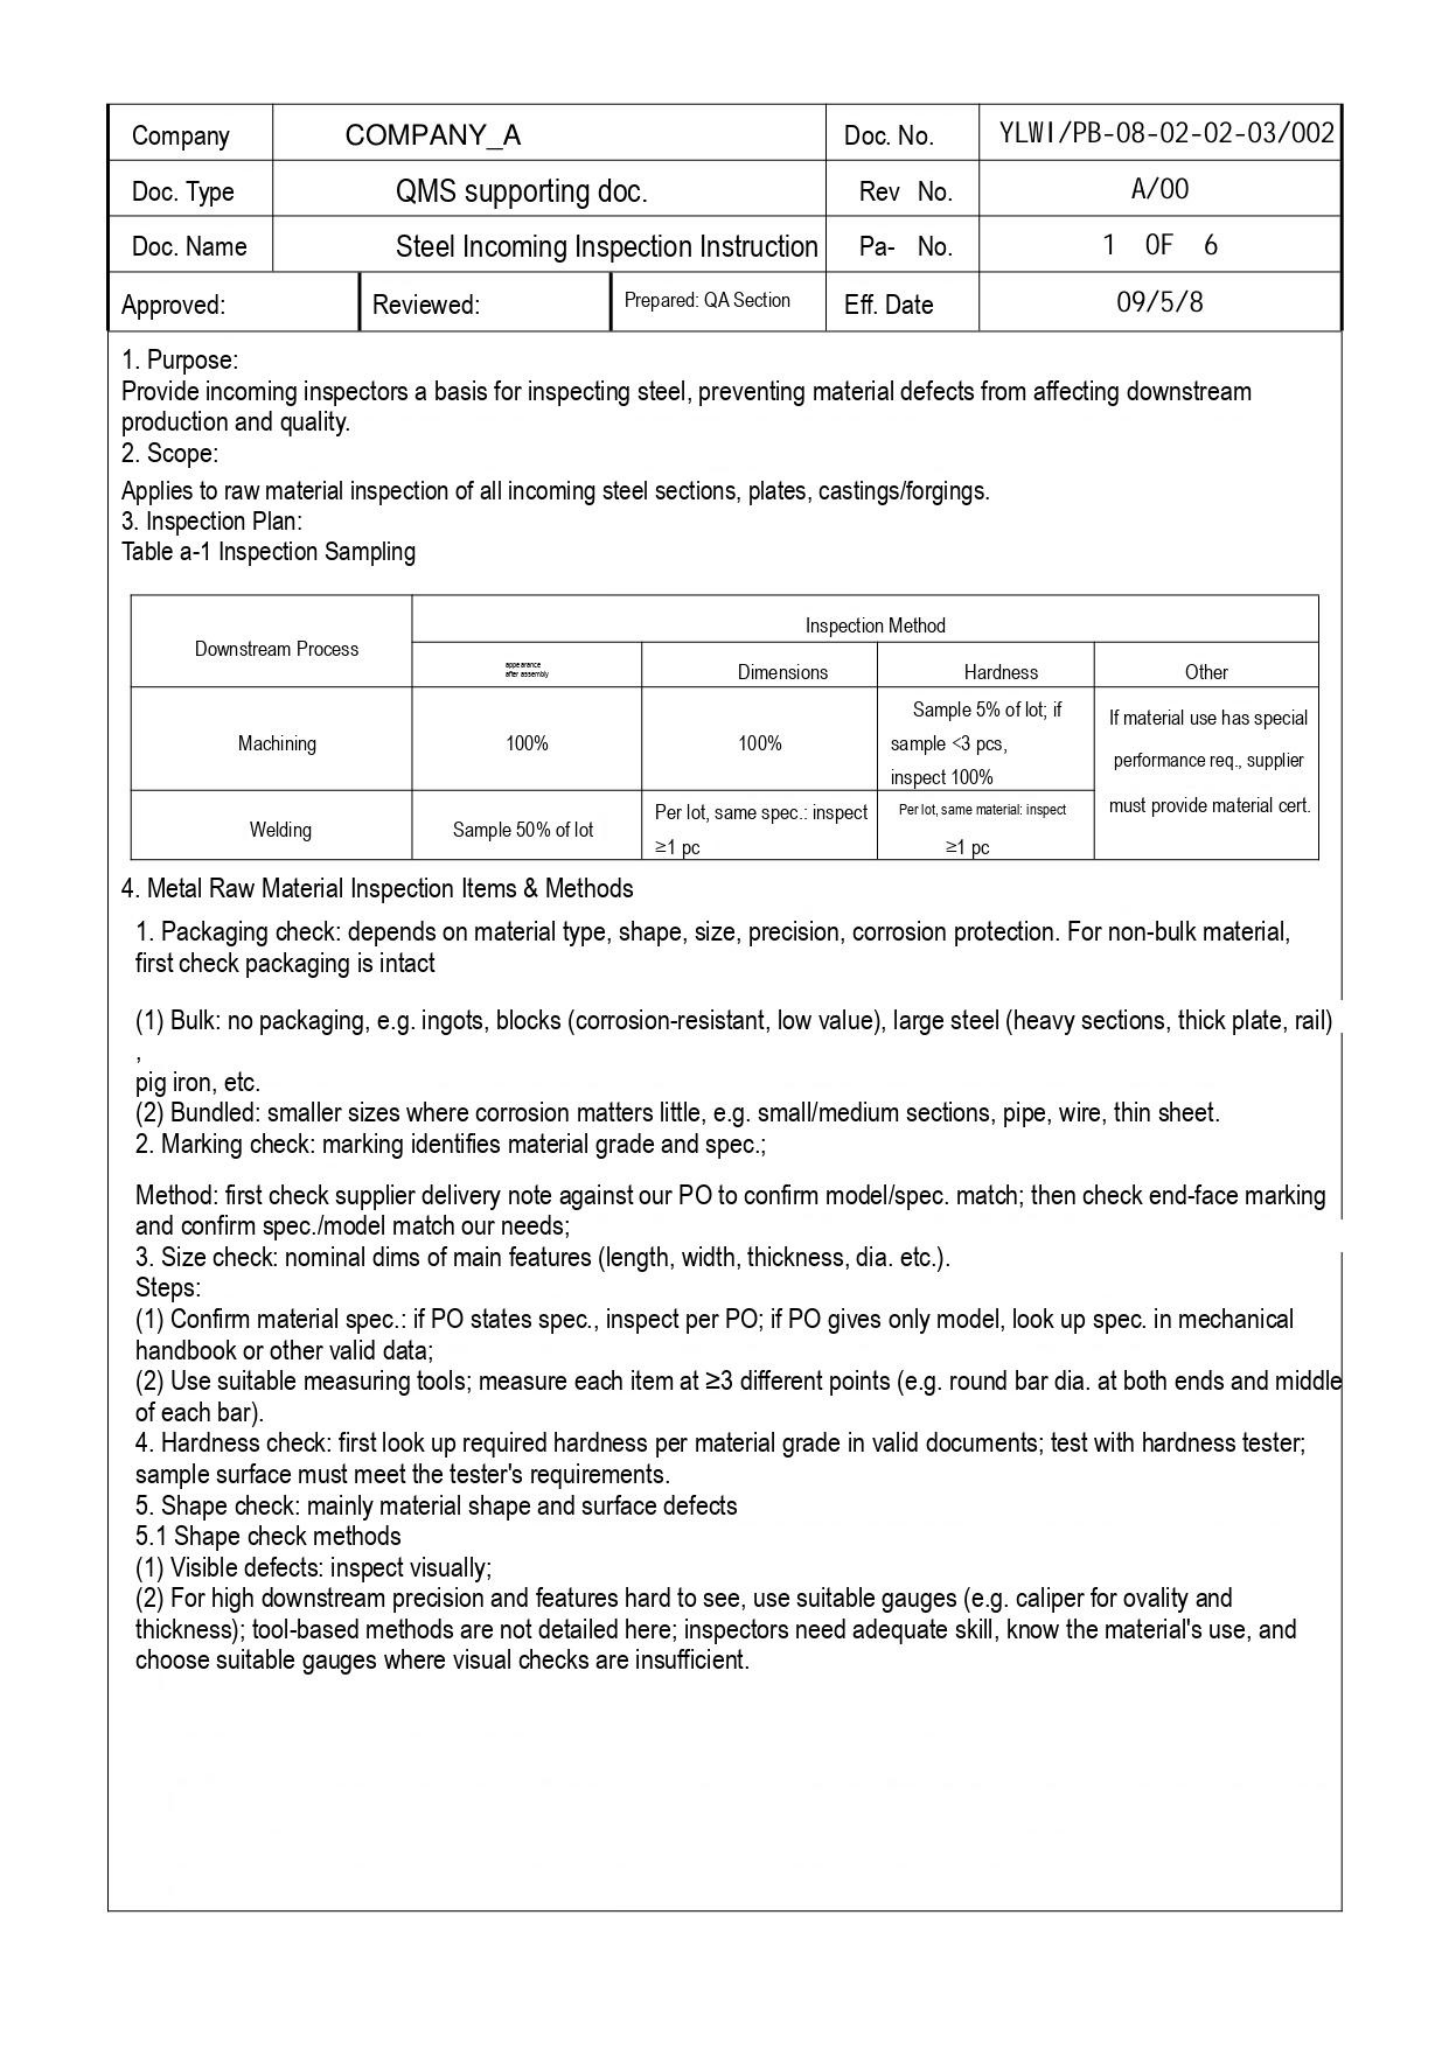| Company | COMPANY_A | | Doc. No. | YLWI/PB-08-02-02-03/002 |
|---|---|---|---|---|
| Doc. Type | QMS supporting doc. | | Rev No. | A/00 |
| Doc. Name | Steel Incoming Inspection Instruction | | Pa- No. | 1 OF 6 |
| Approved: | Reviewed: | Prepared: QA Section | Eff. Date | 09/5/8 |

1. Purpose:
Provide incoming inspectors a basis for inspecting steel, preventing material defects from affecting downstream production and quality.
2. Scope:
Applies to raw material inspection of all incoming steel sections, plates, castings/forgings.
3. Inspection Plan:
Table a-1 Inspection Sampling

| Downstream Process | Inspection Method | | | |
|---|---|---|---|---|
| | appearance after assembly | Dimensions | Hardness | Other |
| Machining | 100% | 100% | Sample 5% of lot; if sample <3 pcs, inspect 100% | If material use has special performance req., supplier must provide material cert. |
| Welding | Sample 50% of lot | Per lot, same spec.: inspect ≥1 pc | Per lot, same material: inspect ≥1 pc | |

4. Metal Raw Material Inspection Items & Methods
1. Packaging check: depends on material type, shape, size, precision, corrosion protection. For non-bulk material, first check packaging is intact

(1) Bulk: no packaging, e.g. ingots, blocks (corrosion-resistant, low value), large steel (heavy sections, thick plate, rail)
,
pig iron, etc.
(2) Bundled: smaller sizes where corrosion matters little, e.g. small/medium sections, pipe, wire, thin sheet.
2. Marking check: marking identifies material grade and spec.;

Method: first check supplier delivery note against our PO to confirm model/spec. match; then check end-face marking and confirm spec./model match our needs;
3. Size check: nominal dims of main features (length, width, thickness, dia. etc.).
Steps:
(1) Confirm material spec.: if PO states spec., inspect per PO; if PO gives only model, look up spec. in mechanical handbook or other valid data;
(2) Use suitable measuring tools; measure each item at ≥3 different points (e.g. round bar dia. at both ends and middle of each bar).
4. Hardness check: first look up required hardness per material grade in valid documents; test with hardness tester; sample surface must meet the tester's requirements.
5. Shape check: mainly material shape and surface defects
5.1 Shape check methods
(1) Visible defects: inspect visually;
(2) For high downstream precision and features hard to see, use suitable gauges (e.g. caliper for ovality and thickness); tool-based methods are not detailed here; inspectors need adequate skill, know the material's use, and choose suitable gauges where visual checks are insufficient.
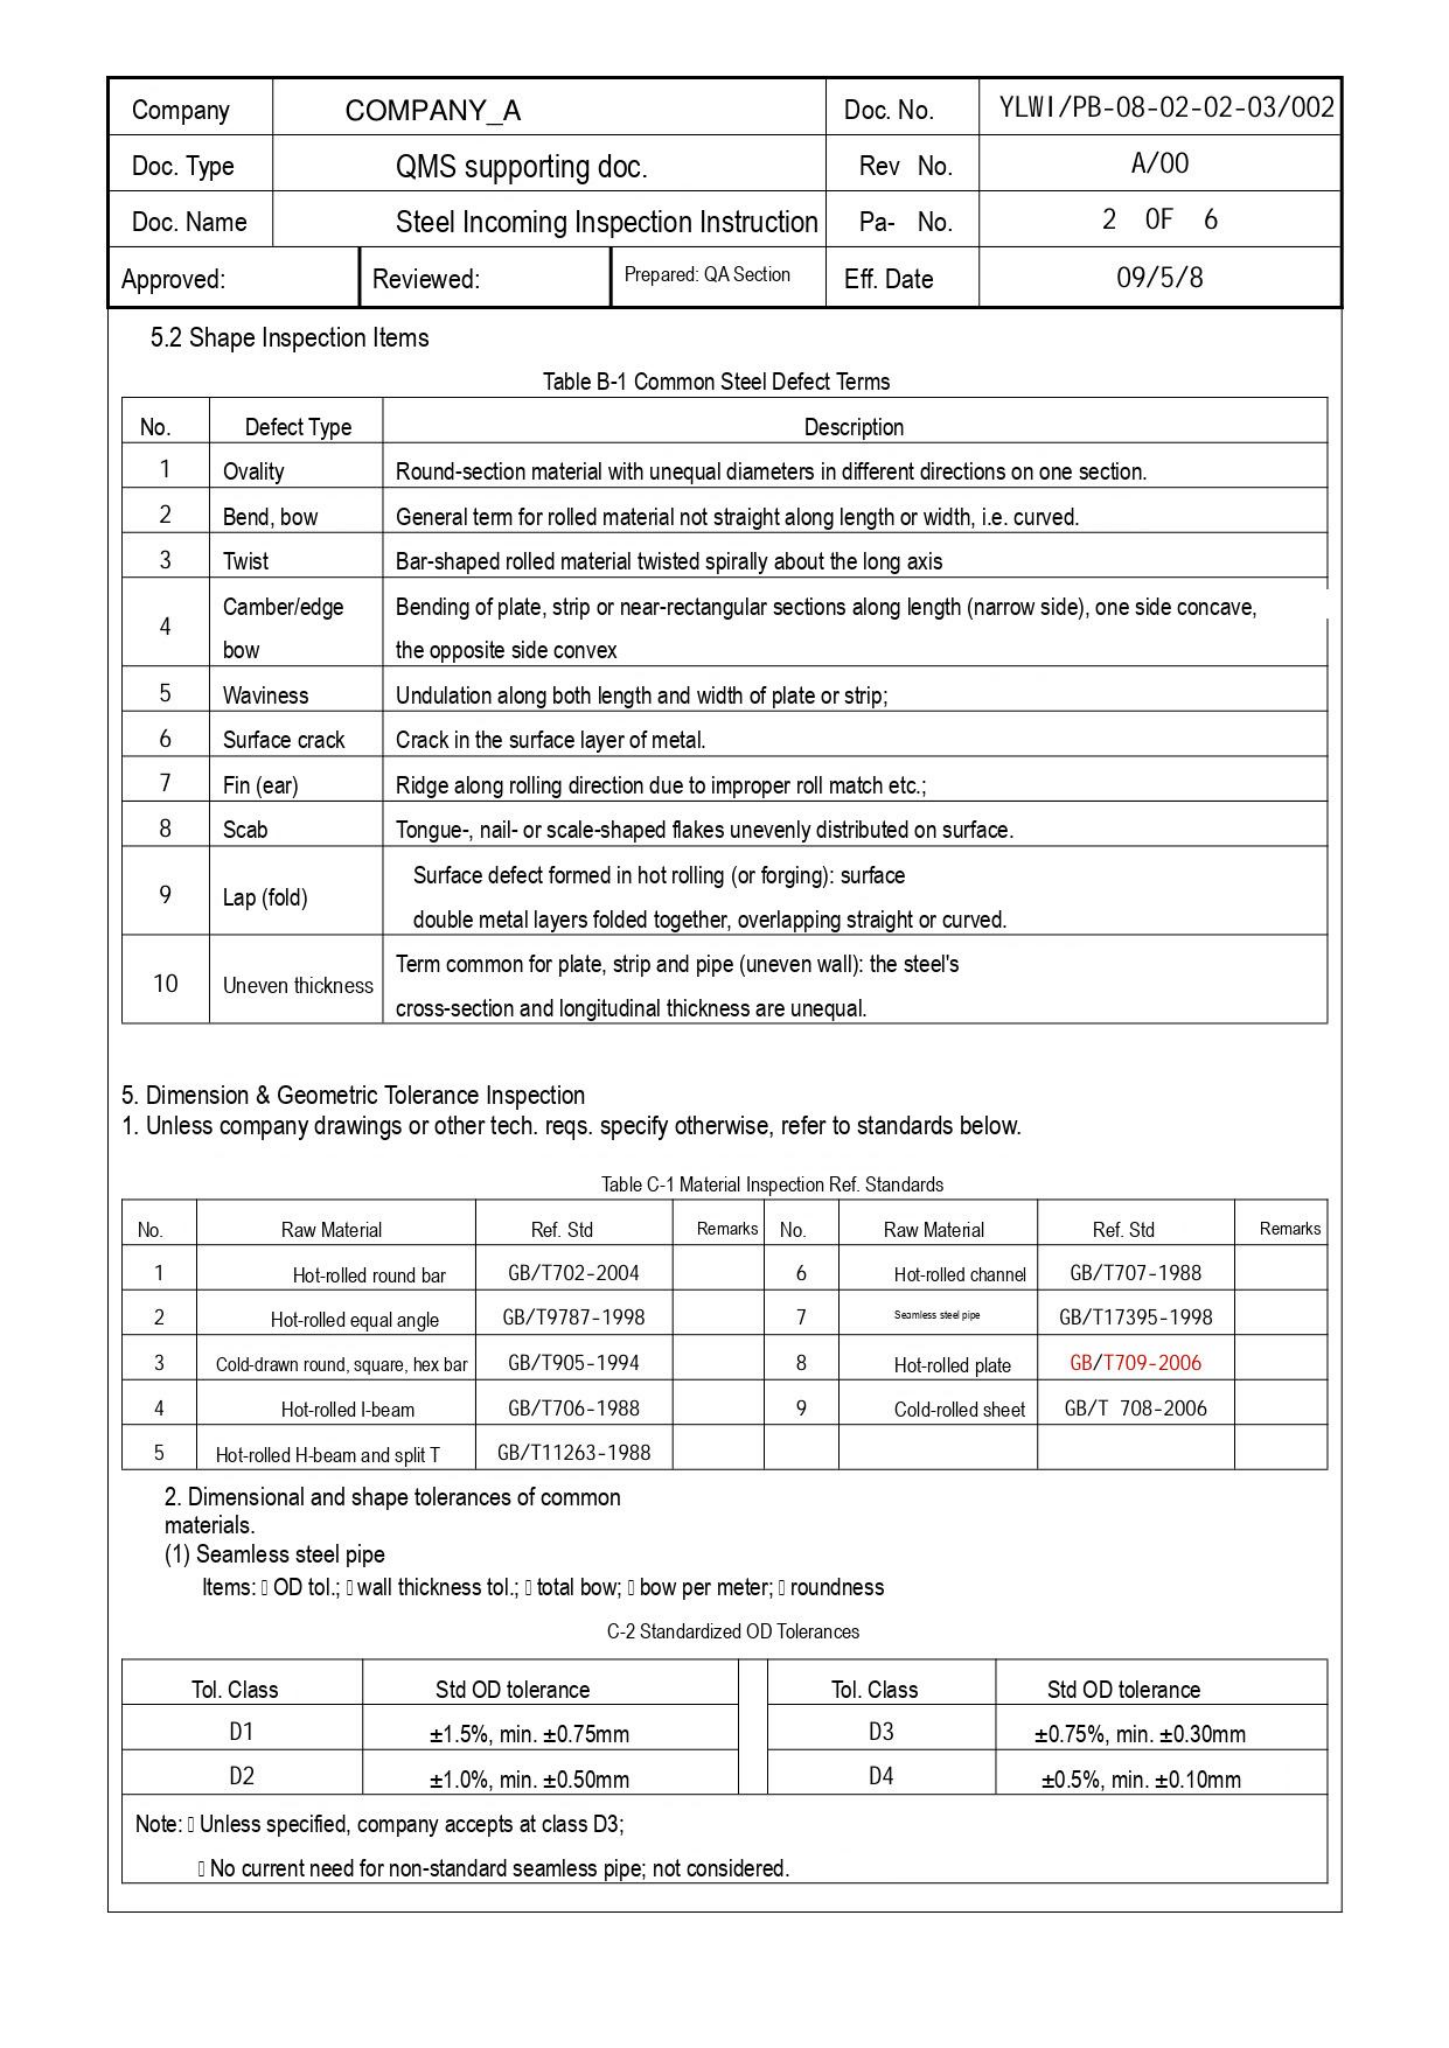| Company | COMPANY_A | Doc. No. | YLWI/PB-08-02-02-03/002 |
|---|---|---|---|
| Doc. Type | QMS supporting doc. | Rev No. | A/00 |
| Doc. Name | Steel Incoming Inspection Instruction | Pa- No. | 2 OF 6 |

| Approved: | Reviewed: | Prepared: QA Section | Eff. Date | 09/5/8 |
|---|---|---|---|---|

5.2 Shape Inspection Items

Table B-1 Common Steel Defect Terms

| No. | Defect Type | Description |
|---|---|---|
| 1 | Ovality | Round-section material with unequal diameters in different directions on one section. |
| 2 | Bend, bow | General term for rolled material not straight along length or width, i.e. curved. |
| 3 | Twist | Bar-shaped rolled material twisted spirally about the long axis |
| 4 | Camber/edge bow | Bending of plate, strip or near-rectangular sections along length (narrow side), one side concave, the opposite side convex |
| 5 | Waviness | Undulation along both length and width of plate or strip; |
| 6 | Surface crack | Crack in the surface layer of metal. |
| 7 | Fin (ear) | Ridge along rolling direction due to improper roll match etc.; |
| 8 | Scab | Tongue-, nail- or scale-shaped flakes unevenly distributed on surface. |
| 9 | Lap (fold) | Surface defect formed in hot rolling (or forging): surface double metal layers folded together, overlapping straight or curved. |
| 10 | Uneven thickness | Term common for plate, strip and pipe (uneven wall): the steel's cross-section and longitudinal thickness are unequal. |

5. Dimension & Geometric Tolerance Inspection
1. Unless company drawings or other tech. reqs. specify otherwise, refer to standards below.

Table C-1 Material Inspection Ref. Standards

| No. | Raw Material | Ref. Std | Remarks | No. | Raw Material | Ref. Std | Remarks |
|---|---|---|---|---|---|---|---|
| 1 | Hot-rolled round bar | GB/T702-2004 | | 6 | Hot-rolled channel | GB/T707-1988 | |
| 2 | Hot-rolled equal angle | GB/T9787-1998 | | 7 | Seamless steel pipe | GB/T17395-1998 | |
| 3 | Cold-drawn round, square, hex bar | GB/T905-1994 | | 8 | Hot-rolled plate | GB/T709-2006 | |
| 4 | Hot-rolled I-beam | GB/T706-1988 | | 9 | Cold-rolled sheet | GB/T 708-2006 | |
| 5 | Hot-rolled H-beam and split T | GB/T11263-1988 | | | | | |

2. Dimensional and shape tolerances of common materials.
(1) Seamless steel pipe
Items: OD tol.; wall thickness tol.; total bow; bow per meter; roundness

C-2 Standardized OD Tolerances

| Tol. Class | Std OD tolerance | Tol. Class | Std OD tolerance |
|---|---|---|---|
| D1 | ±1.5%, min. ±0.75mm | D3 | ±0.75%, min. ±0.30mm |
| D2 | ±1.0%, min. ±0.50mm | D4 | ±0.5%, min. ±0.10mm |

Note: Unless specified, company accepts at class D3;
No current need for non-standard seamless pipe; not considered.
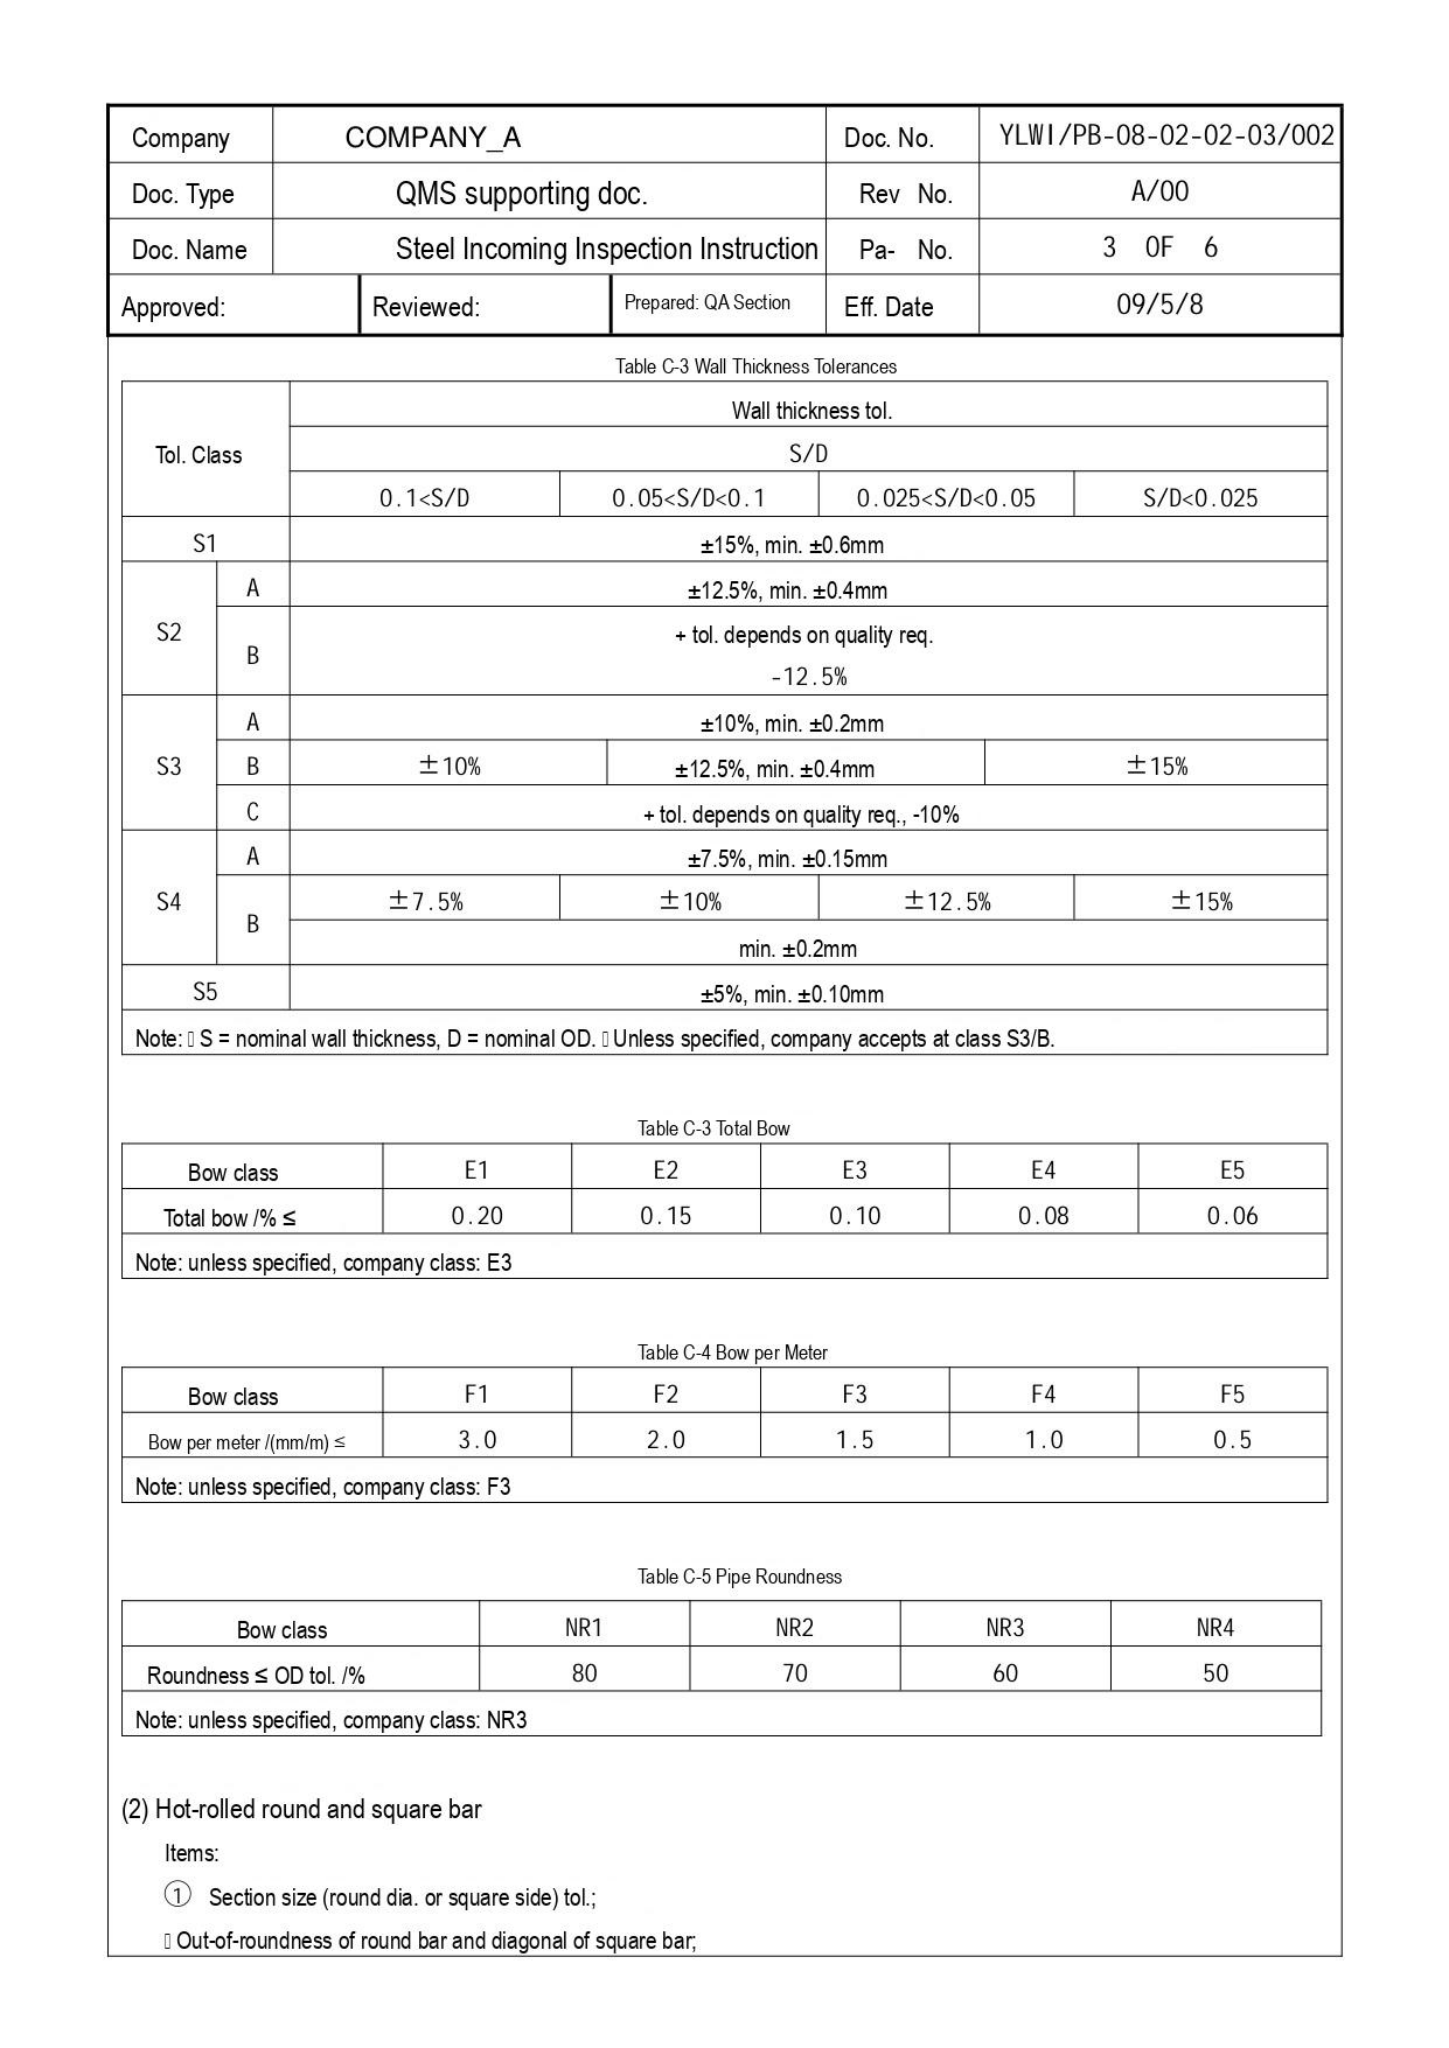| Company | COMPANY_A | | Doc. No. | YLWI/PB-08-02-02-03/002 |
|---|---|---|---|---|
| Doc. Type | QMS supporting doc. | | Rev No. | A/00 |
| Doc. Name | Steel Incoming Inspection Instruction | | Pa- No. | 3 OF 6 |
| Approved: | Reviewed: | Prepared: QA Section | Eff. Date | 09/5/8 |

Table C-3 Wall Thickness Tolerances

| Tol. Class | | Wall thickness tol. | | | |
|---|---|---|---|---|---|
| | | S/D | | | |
| | | 0.1<S/D | 0.05<S/D<0.1 | 0.025<S/D<0.05 | S/D<0.025 |
| S1 | | ±15%, min. ±0.6mm | | | |
| S2 | A | ±12.5%, min. ±0.4mm | | | |
| | B | + tol. depends on quality req.<br>-12.5% | | | |
| S3 | A | ±10%, min. ±0.2mm | | | |
| | B | ±10% | ±12.5%, min. ±0.4mm | | ±15% |
| | C | + tol. depends on quality req., -10% | | | |
| S4 | A | ±7.5%, min. ±0.15mm | | | |
| | B | ±7.5% | ±10% | ±12.5% | ±15% |
| | | min. ±0.2mm | | | |
| S5 | | ±5%, min. ±0.10mm | | | |
| Note: S = nominal wall thickness, D = nominal OD. Unless specified, company accepts at class S3/B. | | | | | |

Table C-3 Total Bow

| Bow class | E1 | E2 | E3 | E4 | E5 |
|---|---|---|---|---|---|
| Total bow /% ≤ | 0.20 | 0.15 | 0.10 | 0.08 | 0.06 |
| Note: unless specified, company class: E3 | | | | | |

Table C-4 Bow per Meter

| Bow class | F1 | F2 | F3 | F4 | F5 |
|---|---|---|---|---|---|
| Bow per meter /(mm/m) ≤ | 3.0 | 2.0 | 1.5 | 1.0 | 0.5 |
| Note: unless specified, company class: F3 | | | | | |

Table C-5 Pipe Roundness

| Bow class | NR1 | NR2 | NR3 | NR4 |
|---|---|---|---|---|
| Roundness ≤ OD tol. /% | 80 | 70 | 60 | 50 |
| Note: unless specified, company class: NR3 | | | | |

(2) Hot-rolled round and square bar

Items:

① Section size (round dia. or square side) tol.;

Out-of-roundness of round bar and diagonal of square bar;
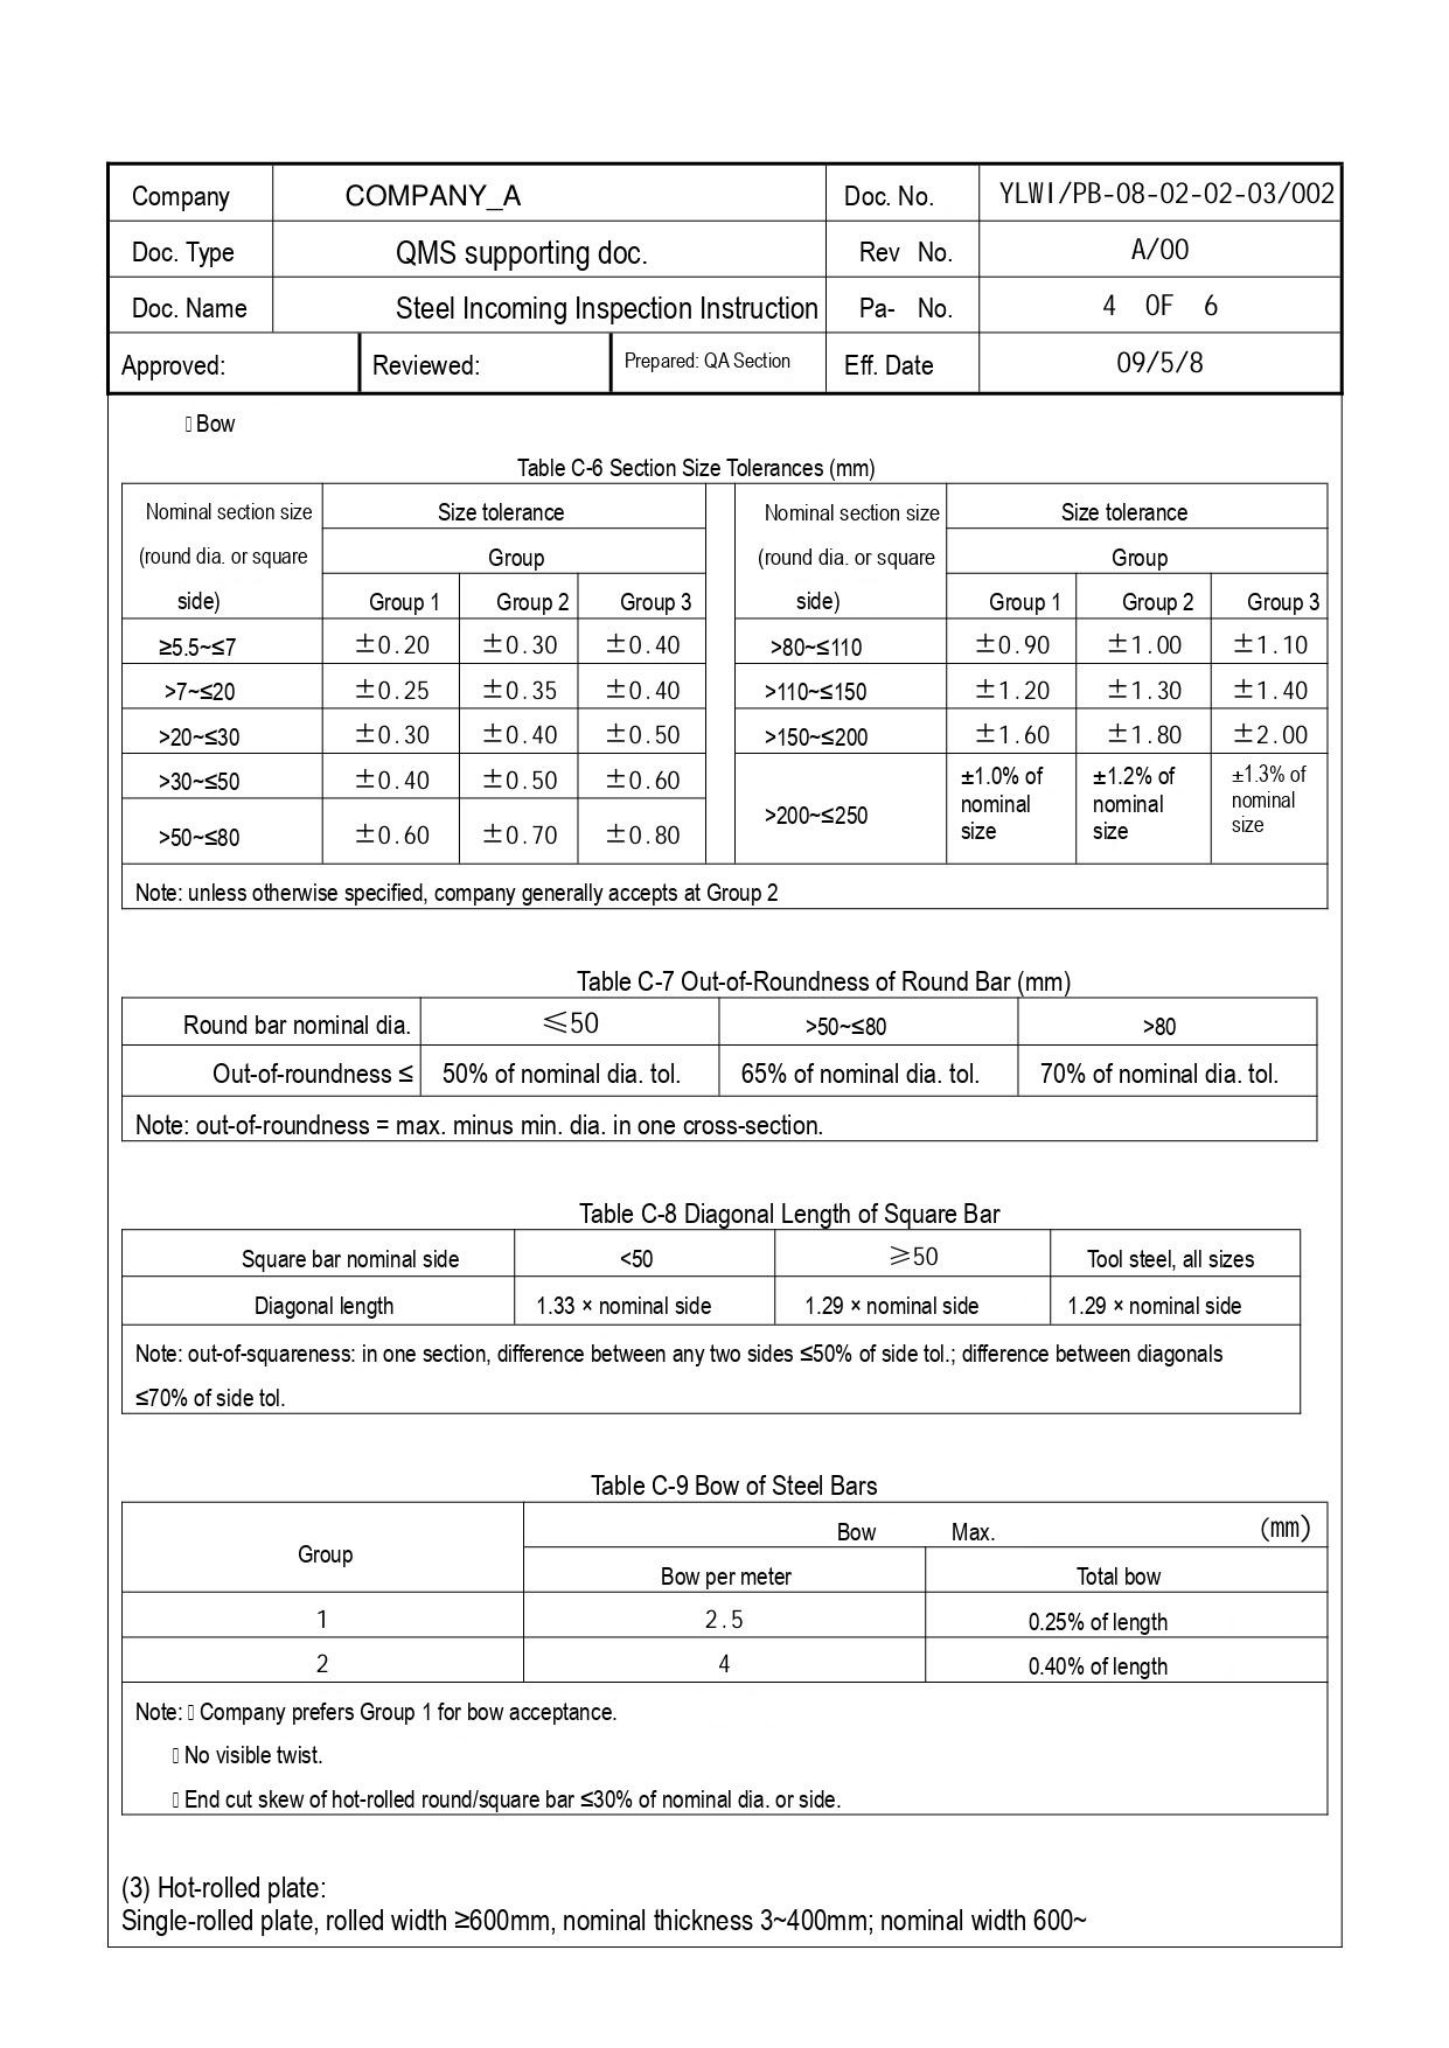| Company | COMPANY_A | | Doc. No. | YLWI/PB-08-02-02-03/002 |
|---|---|---|---|---|
| Doc. Type | QMS supporting doc. | | Rev No. | A/00 |
| Doc. Name | Steel Incoming Inspection Instruction | | Pa- No. | 4 OF 6 |
| Approved: | Reviewed: | Prepared: QA Section | Eff. Date | 09/5/8 |

Bow

Table C-6 Section Size Tolerances (mm)

| Nominal section size (round dia. or square side) | Size tolerance Group Group 1 | Size tolerance Group Group 2 | Size tolerance Group Group 3 | Nominal section size (round dia. or square side) | Size tolerance Group Group 1 | Size tolerance Group Group 2 | Size tolerance Group Group 3 |
|---|---|---|---|---|---|---|---|
| ≥5.5~≤7 | ±0.20 | ±0.30 | ±0.40 | >80~≤110 | ±0.90 | ±1.00 | ±1.10 |
| >7~≤20 | ±0.25 | ±0.35 | ±0.40 | >110~≤150 | ±1.20 | ±1.30 | ±1.40 |
| >20~≤30 | ±0.30 | ±0.40 | ±0.50 | >150~≤200 | ±1.60 | ±1.80 | ±2.00 |
| >30~≤50 | ±0.40 | ±0.50 | ±0.60 | >200~≤250 | ±1.0% of nominal size | ±1.2% of nominal size | ±1.3% of nominal size |
| >50~≤80 | ±0.60 | ±0.70 | ±0.80 | | | | |
| Note: unless otherwise specified, company generally accepts at Group 2 | | | | | | | |

Table C-7 Out-of-Roundness of Round Bar (mm)

| Round bar nominal dia. | ≤50 | >50~≤80 | >80 |
|---|---|---|---|
| Out-of-roundness ≤ | 50% of nominal dia. tol. | 65% of nominal dia. tol. | 70% of nominal dia. tol. |
| Note: out-of-roundness = max. minus min. dia. in one cross-section. | | | |

Table C-8 Diagonal Length of Square Bar

| Square bar nominal side | <50 | ≥50 | Tool steel, all sizes |
|---|---|---|---|
| Diagonal length | 1.33 × nominal side | 1.29 × nominal side | 1.29 × nominal side |
| Note: out-of-squareness: in one section, difference between any two sides ≤50% of side tol.; difference between diagonals ≤70% of side tol. | | | |

Table C-9 Bow of Steel Bars

| Group | Bow Max. (mm) Bow per meter | Bow Max. (mm) Total bow |
|---|---|---|
| 1 | 2.5 | 0.25% of length |
| 2 | 4 | 0.40% of length |
| Note: Company prefers Group 1 for bow acceptance. No visible twist. End cut skew of hot-rolled round/square bar ≤30% of nominal dia. or side. | | |

(3) Hot-rolled plate:
Single-rolled plate, rolled width ≥600mm, nominal thickness 3~400mm; nominal width 600~
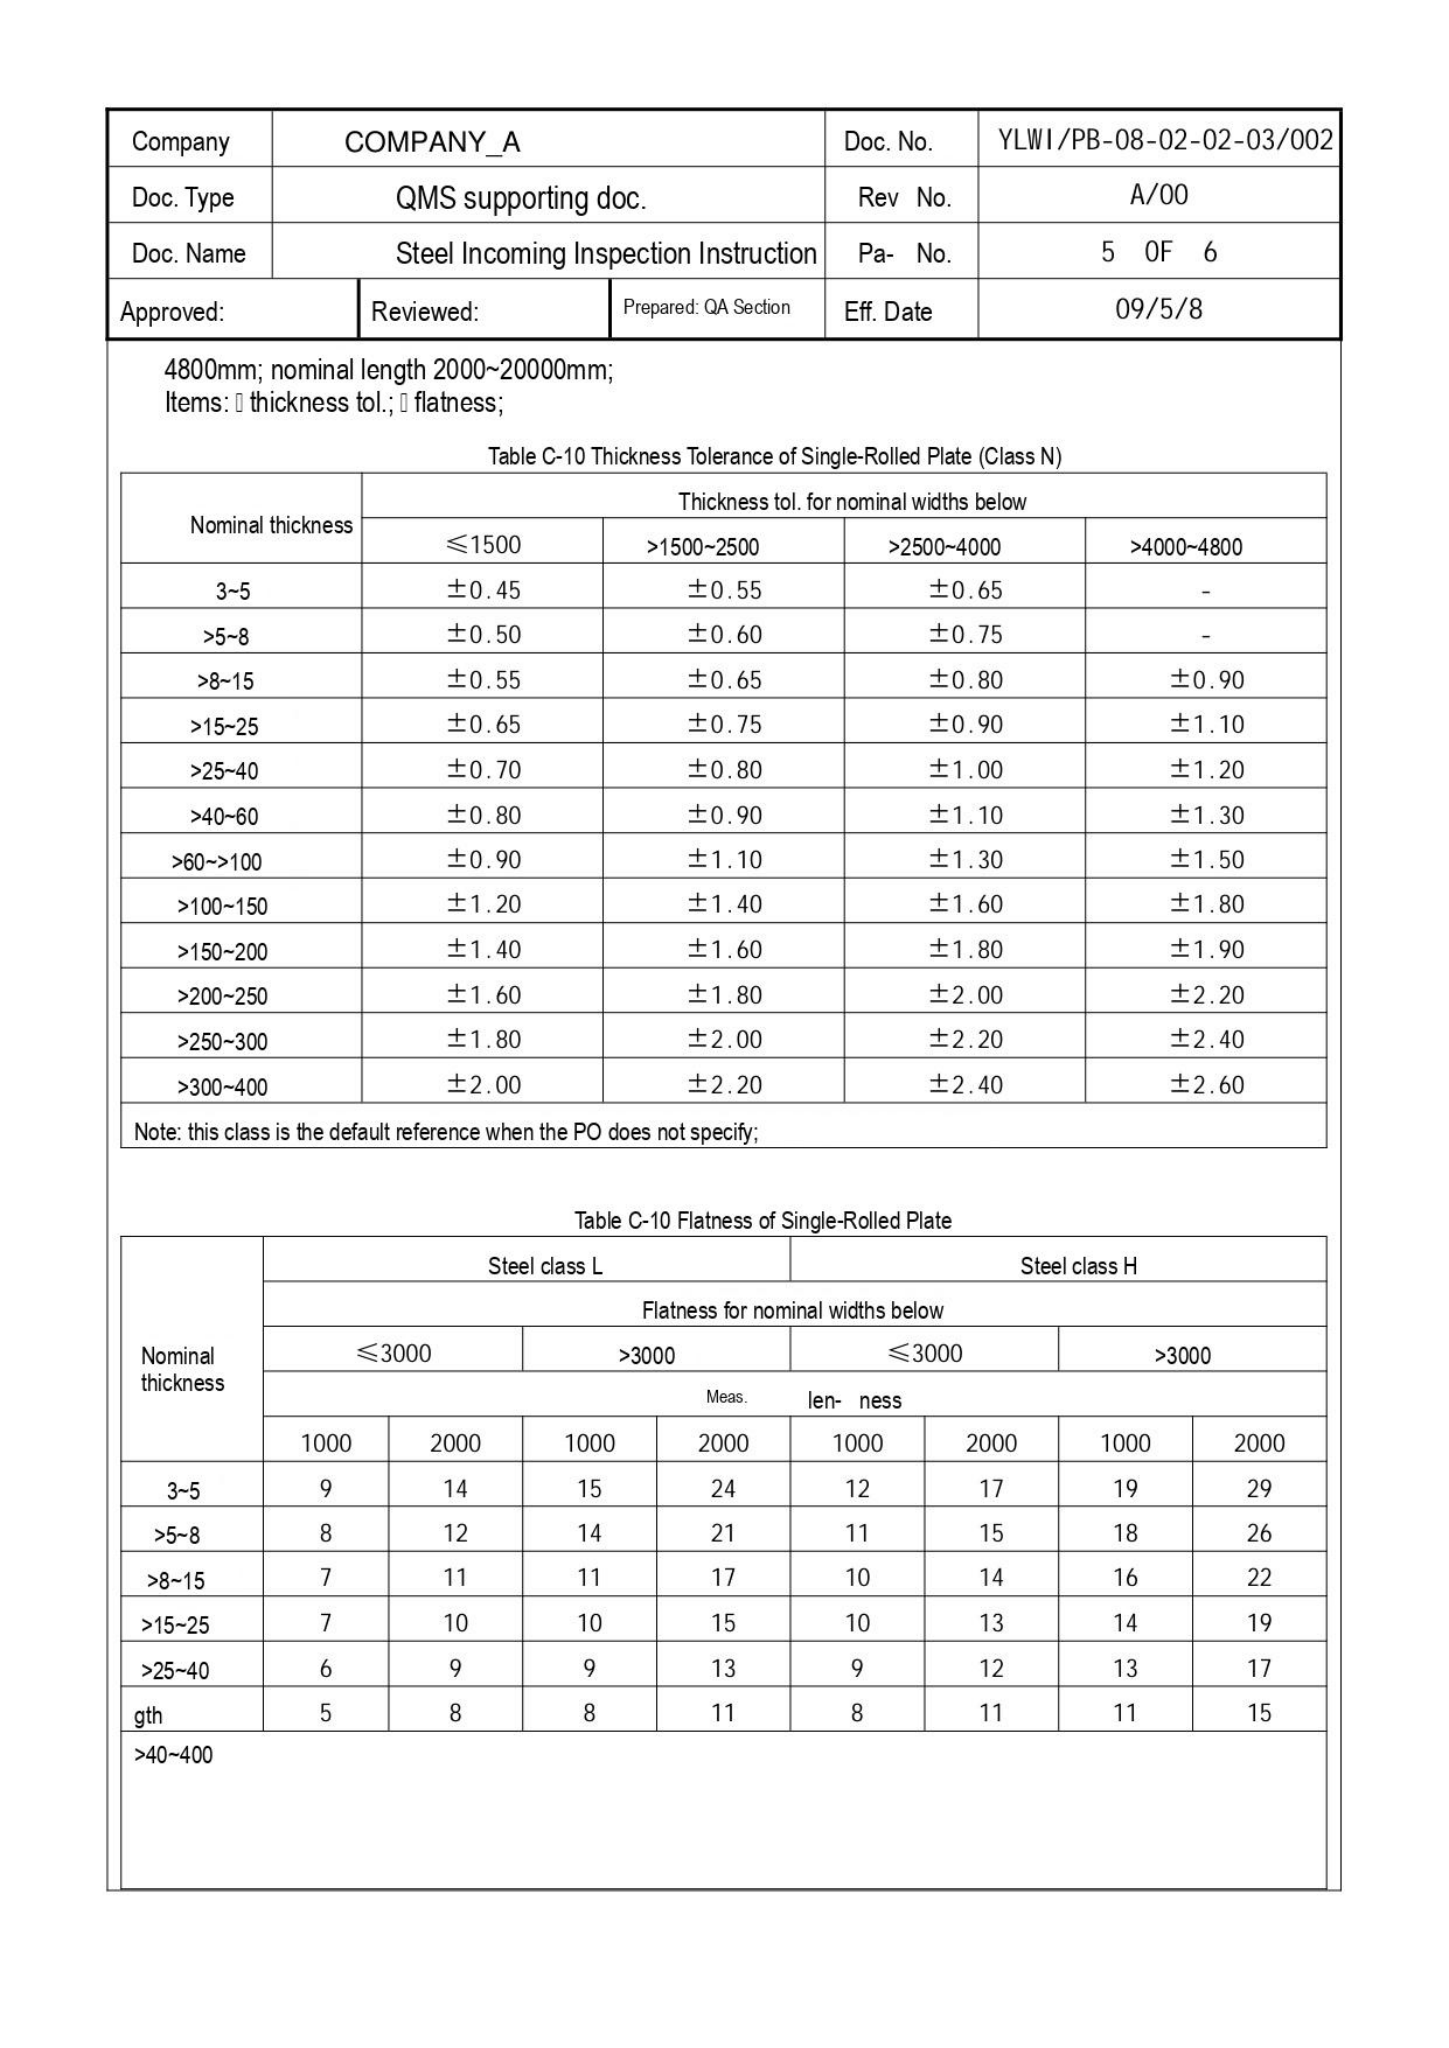| Company | COMPANY_A | | Doc. No. | YLWI/PB-08-02-02-03/002 |
|---|---|---|---|---|
| Doc. Type | QMS supporting doc. | | Rev No. | A/00 |
| Doc. Name | Steel Incoming Inspection Instruction | | Pa- No. | 5 OF 6 |
| Approved: | Reviewed: | Prepared: QA Section | Eff. Date | 09/5/8 |

4800mm; nominal length 2000~20000mm;
Items: thickness tol.; flatness;

Table C-10 Thickness Tolerance of Single-Rolled Plate (Class N)

| Nominal thickness | Thickness tol. for nominal widths below | | | |
|---|---|---|---|---|
| | ≤1500 | >1500~2500 | >2500~4000 | >4000~4800 |
| 3~5 | ±0.45 | ±0.55 | ±0.65 | - |
| >5~8 | ±0.50 | ±0.60 | ±0.75 | - |
| >8~15 | ±0.55 | ±0.65 | ±0.80 | ±0.90 |
| >15~25 | ±0.65 | ±0.75 | ±0.90 | ±1.10 |
| >25~40 | ±0.70 | ±0.80 | ±1.00 | ±1.20 |
| >40~60 | ±0.80 | ±0.90 | ±1.10 | ±1.30 |
| >60~>100 | ±0.90 | ±1.10 | ±1.30 | ±1.50 |
| >100~150 | ±1.20 | ±1.40 | ±1.60 | ±1.80 |
| >150~200 | ±1.40 | ±1.60 | ±1.80 | ±1.90 |
| >200~250 | ±1.60 | ±1.80 | ±2.00 | ±2.20 |
| >250~300 | ±1.80 | ±2.00 | ±2.20 | ±2.40 |
| >300~400 | ±2.00 | ±2.20 | ±2.40 | ±2.60 |
| Note: this class is the default reference when the PO does not specify; | | | | |

Table C-10 Flatness of Single-Rolled Plate

| Nominal thickness | Steel class L | | | | Steel class H | | | |
|---|---|---|---|---|---|---|---|---|
| | Flatness for nominal widths below | | | | | | | |
| | ≤3000 | | >3000 | | ≤3000 | | >3000 | |
| | Meas. len- ness | | | | | | | |
| | 1000 | 2000 | 1000 | 2000 | 1000 | 2000 | 1000 | 2000 |
| 3~5 | 9 | 14 | 15 | 24 | 12 | 17 | 19 | 29 |
| >5~8 | 8 | 12 | 14 | 21 | 11 | 15 | 18 | 26 |
| >8~15 | 7 | 11 | 11 | 17 | 10 | 14 | 16 | 22 |
| >15~25 | 7 | 10 | 10 | 15 | 10 | 13 | 14 | 19 |
| >25~40 | 6 | 9 | 9 | 13 | 9 | 12 | 13 | 17 |
| gth | 5 | 8 | 8 | 11 | 8 | 11 | 11 | 15 |

>40~400
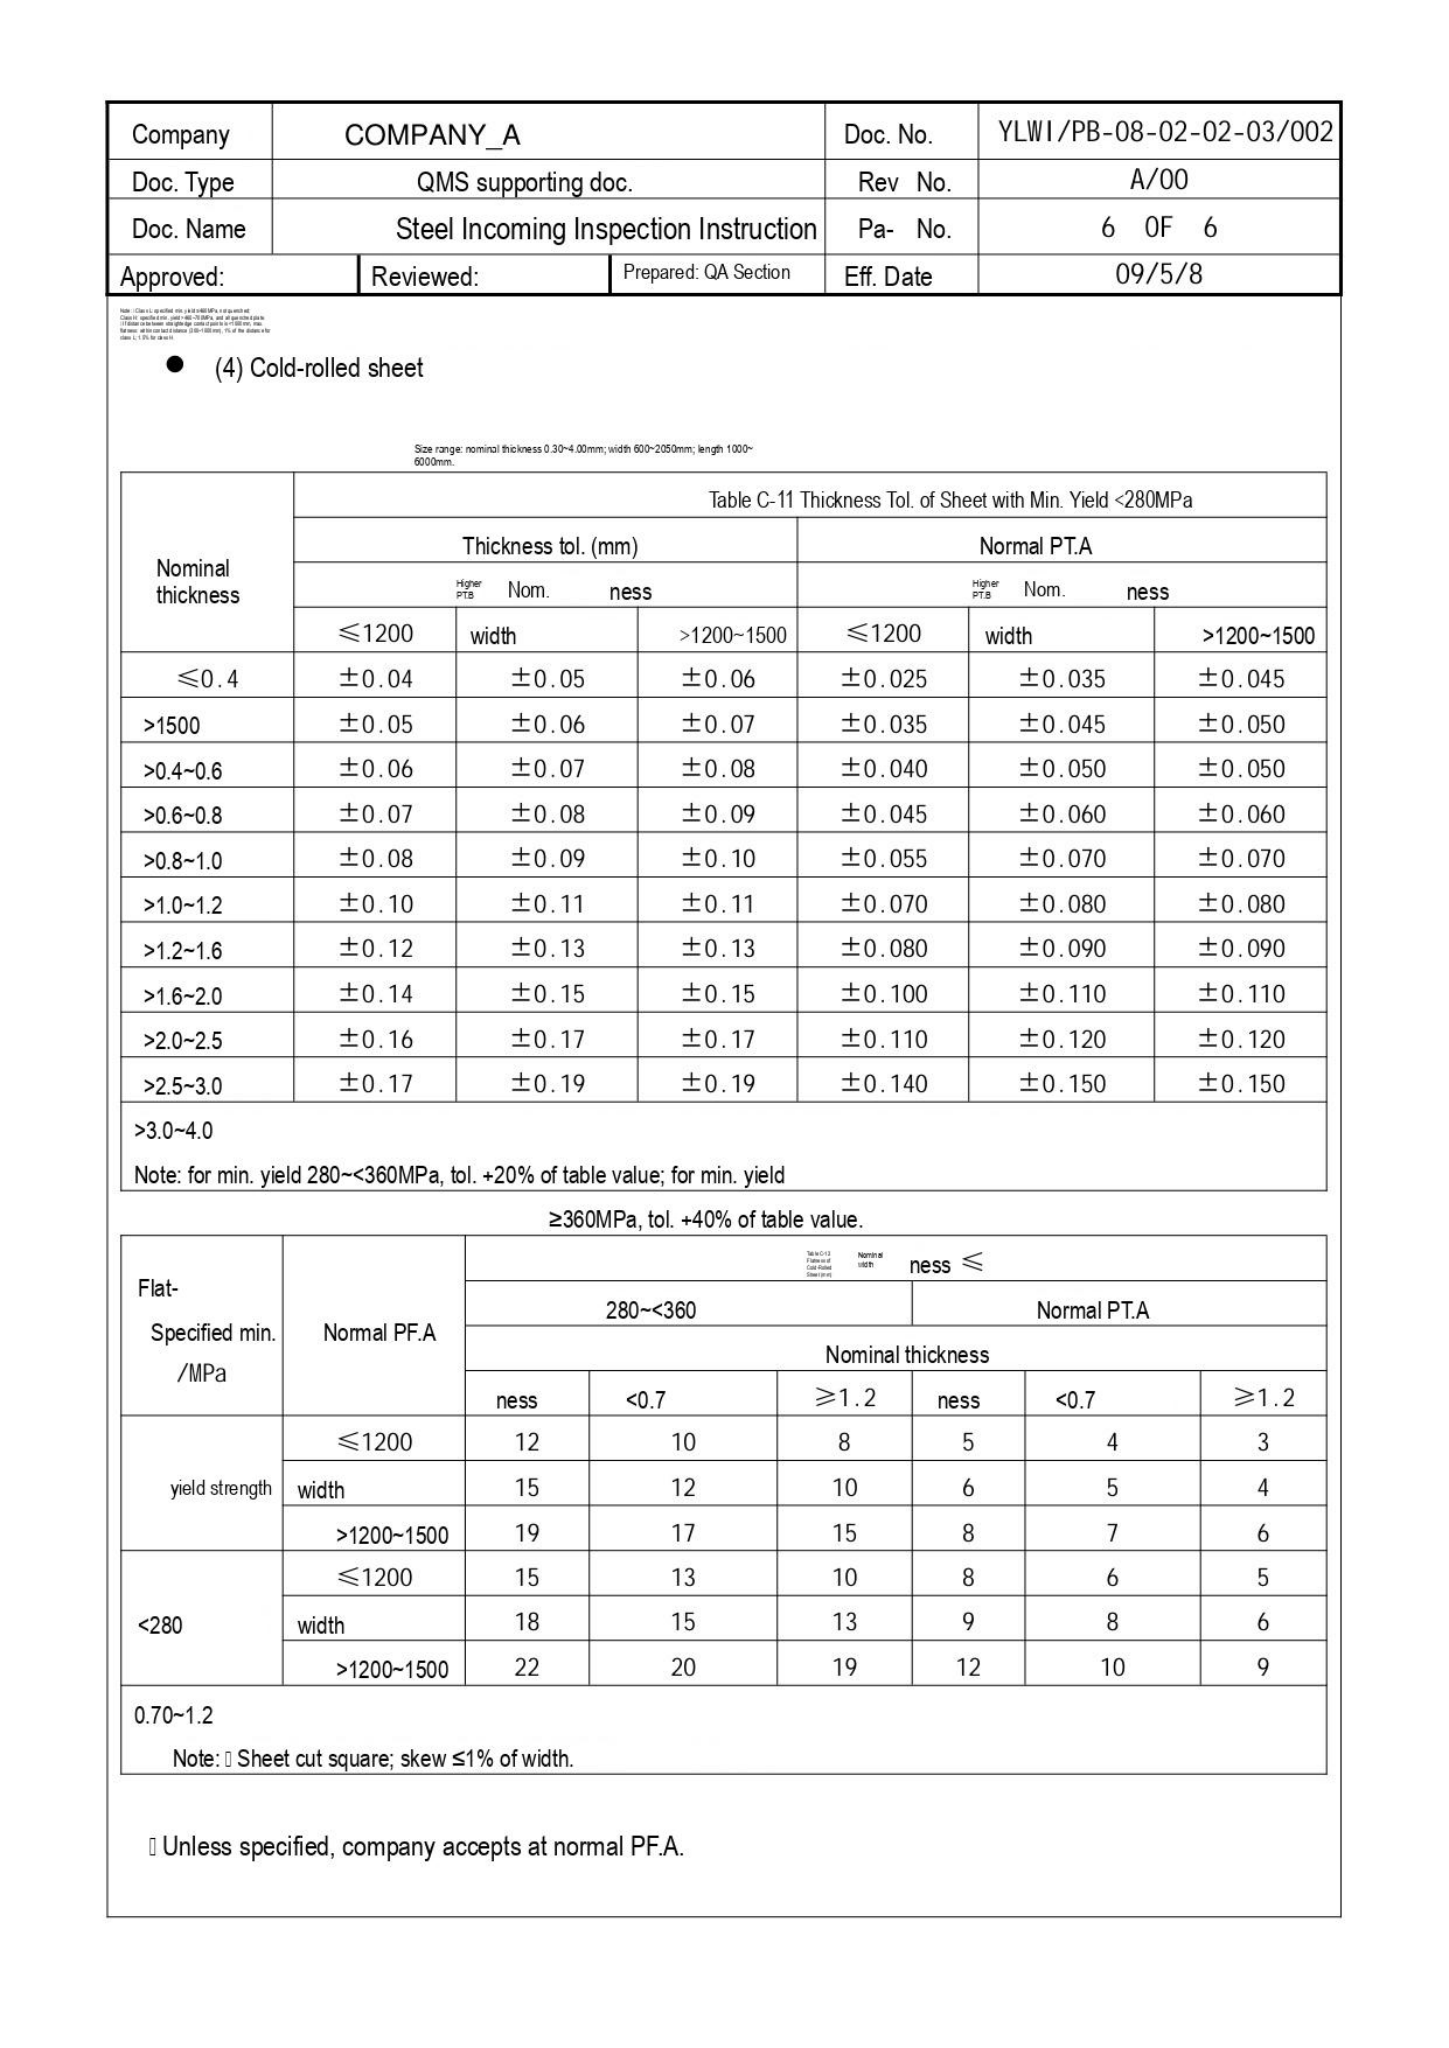| Company | COMPANY_A | Doc. No. | YLWI/PB-08-02-02-03/002 |
|---|---|---|---|
| Doc. Type | QMS supporting doc. | Rev No. | A/00 |
| Doc. Name | Steel Incoming Inspection Instruction | Pa- No. | 6 OF 6 |
| Approved: Reviewed: | Prepared: QA Section | Eff. Date | 09/5/8 |

- (4) Cold-rolled sheet

Size range: nominal thickness 0.30~4.00mm; width 600~2050mm; length 1000~6000mm.

<table>
<tr><td rowspan="4">Nominal thickness</td><td colspan="6">Table C-11 Thickness Tol. of Sheet with Min. Yield &lt;280MPa</td></tr>
<tr><td colspan="3">Thickness tol. (mm)</td><td colspan="3">Normal PT.A</td></tr>
<tr><td colspan="3">Higher PTB Nom. ness</td><td colspan="3">Higher PT.B Nom. ness</td></tr>
<tr><td>≤1200</td><td>width</td><td>&gt;1200~1500</td><td>≤1200</td><td>width</td><td>&gt;1200~1500</td></tr>
<tr><td>≤0.4</td><td>±0.04</td><td>±0.05</td><td>±0.06</td><td>±0.025</td><td>±0.035</td><td>±0.045</td></tr>
<tr><td>&gt;1500</td><td>±0.05</td><td>±0.06</td><td>±0.07</td><td>±0.035</td><td>±0.045</td><td>±0.050</td></tr>
<tr><td>&gt;0.4~0.6</td><td>±0.06</td><td>±0.07</td><td>±0.08</td><td>±0.040</td><td>±0.050</td><td>±0.050</td></tr>
<tr><td>&gt;0.6~0.8</td><td>±0.07</td><td>±0.08</td><td>±0.09</td><td>±0.045</td><td>±0.060</td><td>±0.060</td></tr>
<tr><td>&gt;0.8~1.0</td><td>±0.08</td><td>±0.09</td><td>±0.10</td><td>±0.055</td><td>±0.070</td><td>±0.070</td></tr>
<tr><td>&gt;1.0~1.2</td><td>±0.10</td><td>±0.11</td><td>±0.11</td><td>±0.070</td><td>±0.080</td><td>±0.080</td></tr>
<tr><td>&gt;1.2~1.6</td><td>±0.12</td><td>±0.13</td><td>±0.13</td><td>±0.080</td><td>±0.090</td><td>±0.090</td></tr>
<tr><td>&gt;1.6~2.0</td><td>±0.14</td><td>±0.15</td><td>±0.15</td><td>±0.100</td><td>±0.110</td><td>±0.110</td></tr>
<tr><td>&gt;2.0~2.5</td><td>±0.16</td><td>±0.17</td><td>±0.17</td><td>±0.110</td><td>±0.120</td><td>±0.120</td></tr>
<tr><td>&gt;2.5~3.0</td><td>±0.17</td><td>±0.19</td><td>±0.19</td><td>±0.140</td><td>±0.150</td><td>±0.150</td></tr>
<tr><td colspan="7">&gt;3.0~4.0<br>Note: for min. yield 280~&lt;360MPa, tol. +20% of table value; for min. yield</td></tr>
</table>

≥360MPa, tol. +40% of table value.

<table>
<tr><td rowspan="4">Flat-<br>Specified min. /MPa</td><td rowspan="4">Normal PF.A</td><td colspan="6">Table C-12 Flatness of Cold-Rolled Sheet (mm) Nominal width ness ≤</td></tr>
<tr><td colspan="3">280~&lt;360</td><td colspan="3">Normal PT.A</td></tr>
<tr><td colspan="6">Nominal thickness</td></tr>
<tr><td>ness</td><td>&lt;0.7</td><td>≥1.2</td><td>ness</td><td>&lt;0.7</td><td>≥1.2</td></tr>
<tr><td rowspan="3">yield strength</td><td>≤1200</td><td>12</td><td>10</td><td>8</td><td>5</td><td>4</td><td>3</td></tr>
<tr><td>width</td><td>15</td><td>12</td><td>10</td><td>6</td><td>5</td><td>4</td></tr>
<tr><td>&gt;1200~1500</td><td>19</td><td>17</td><td>15</td><td>8</td><td>7</td><td>6</td></tr>
<tr><td rowspan="3">&lt;280</td><td>≤1200</td><td>15</td><td>13</td><td>10</td><td>8</td><td>6</td><td>5</td></tr>
<tr><td>width</td><td>18</td><td>15</td><td>13</td><td>9</td><td>8</td><td>6</td></tr>
<tr><td>&gt;1200~1500</td><td>22</td><td>20</td><td>19</td><td>12</td><td>10</td><td>9</td></tr>
<tr><td colspan="8">0.70~1.2<br>Note: Sheet cut square; skew ≤1% of width.</td></tr>
</table>

Unless specified, company accepts at normal PF.A.